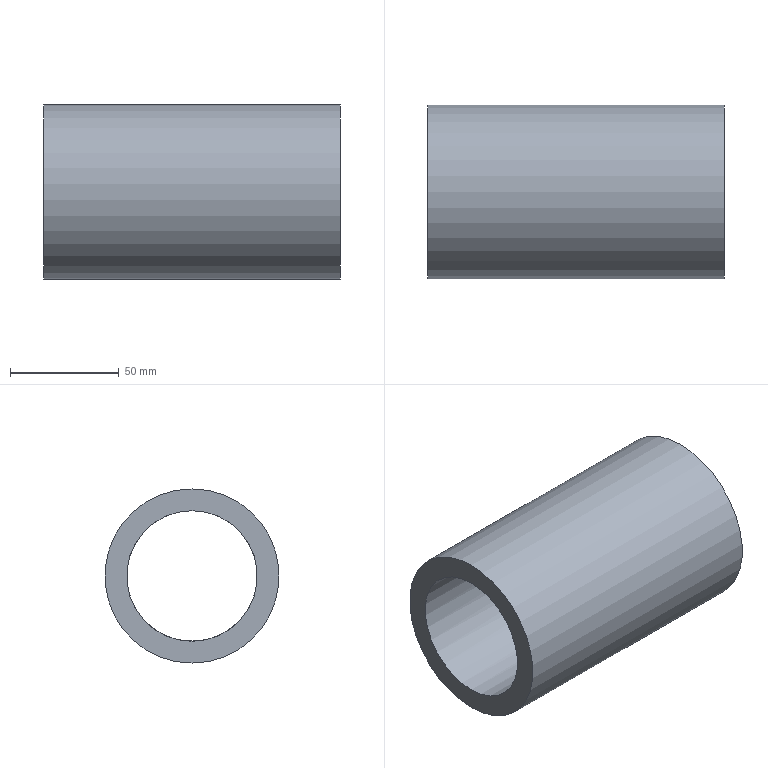Part | STEP file | solid 158 | 1 solid | 4 faces | box 136 x 80 x 80 mm | volume 299080 mm3 | plane 2 | cylinder 2 | commonest cylinder face diameters 60 x1 80 x1